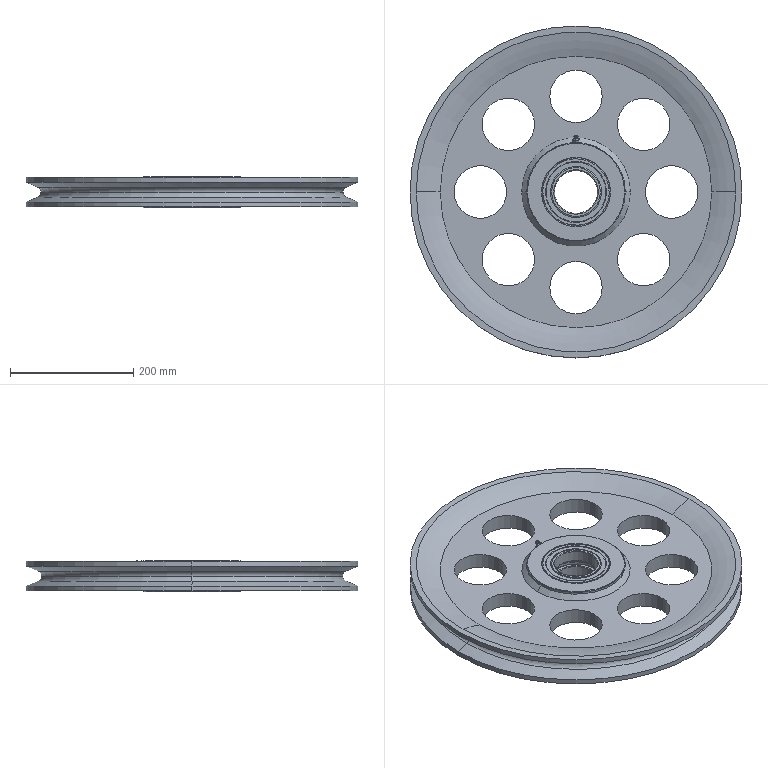Part | SolidWorks | 52 solids | 653 faces | box 538 x 538 x 50.446 mm | volume 5101431 mm3 | cylinder 252 | sphere 192 | plane 129 | torus 52 | cone 28 | commonest cylinder face diameters 88 x90 92 x90 85 x16 83.333 x8 96.667 x8 110 x8